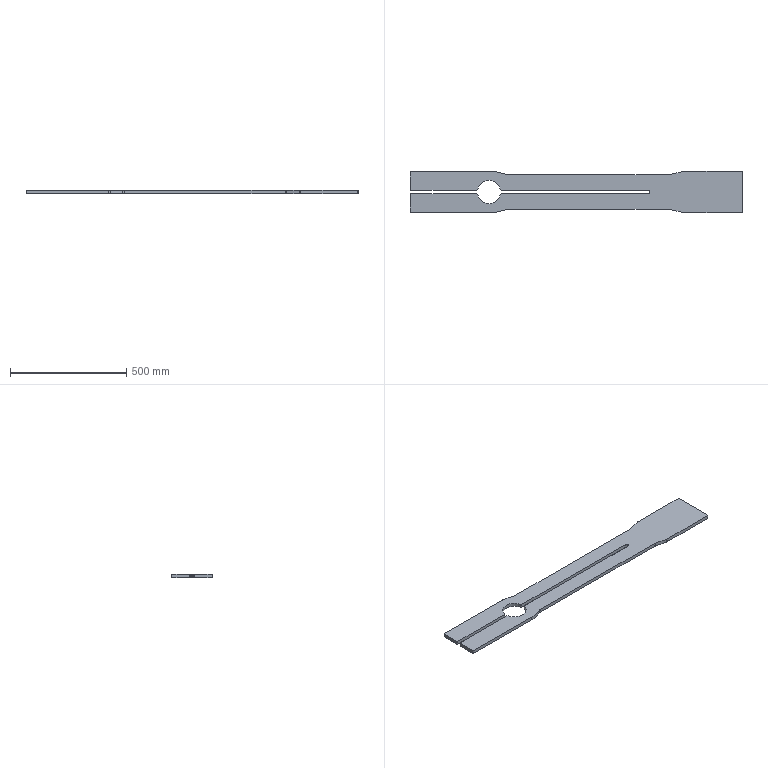Part | STEP file | Planar support platform panel | 1 solid | 42 faces | box 1430 x 180 x 15 mm | volume 3191288 mm3 | plane 30 | cylinder 12 | commonest cylinder face diameters 60 x8 10 x2 100 x2